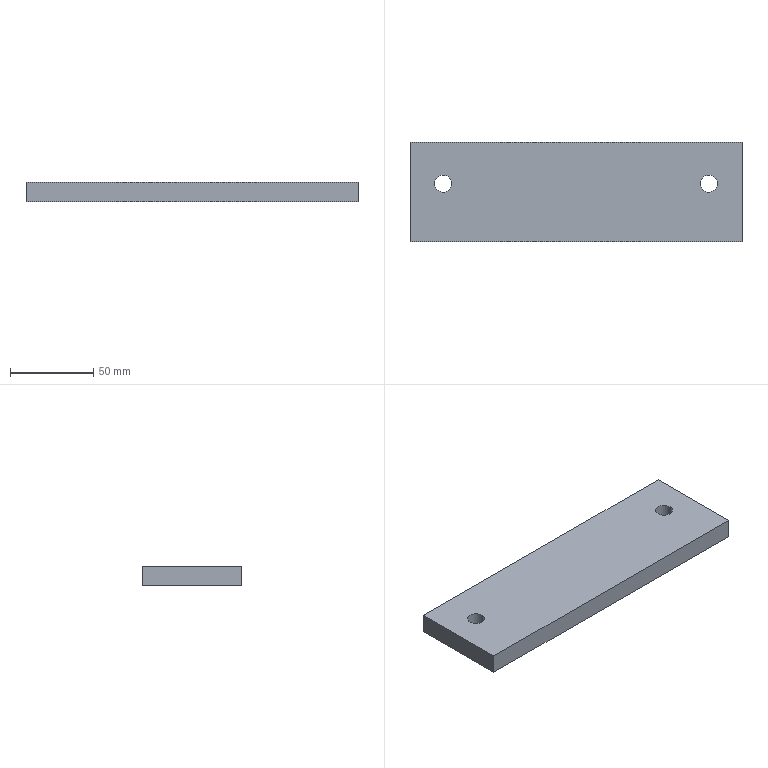Part | SolidWorks | features Extrusion 1, HoleWzd 1 | 1 solid | 10 faces | box 200 x 60 x 12 mm | volume 142039 mm3 | plane 6 | cylinder 4 | commonest cylinder face diameters 10.2 x4
STEP:
#1=CARTESIAN_POINT('',(-85.1,5.,0.));
#2=VERTEX_POINT('',#1);
#3=CARTESIAN_POINT('',(-74.9,5.,0.));
#4=VERTEX_POINT('',#3);
#5=CARTESIAN_POINT('',(-80.,5.,0.));
#6=DIRECTION('',(0.,0.,1.));
#7=DIRECTION('',(1.,0.,0.));
#8=AXIS2_PLACEMENT_3D('',#5,#6,#7);
#9=CIRCLE('',#8,5.1);
#10=EDGE_CURVE('',#2,#4,#9,.T.);
#11=ORIENTED_EDGE('',*,*,#10,.F.);
#12=CARTESIAN_POINT('',(-85.1,5.,12.));
#13=VERTEX_POINT('',#12);
#14=CARTESIAN_POINT('',(-85.1,5.,12.));
#15=DIRECTION('',(0.,0.,1.));
#16=VECTOR('',#15,1000.);
#17=LINE('',#14,#16);
#18=EDGE_CURVE('',#2,#13,#17,.T.);
#19=ORIENTED_EDGE('',*,*,#18,.T.);
#20=CARTESIAN_POINT('',(-74.9,5.,12.));
#21=VERTEX_POINT('',#20);
#22=CARTESIAN_POINT('',(-80.,5.,12.));
#23=DIRECTION('',(0.,0.,1.));
#24=DIRECTION('',(1.,0.,0.));
#25=AXIS2_PLACEMENT_3D('',#22,#23,#24);
#26=CIRCLE('',#25,5.1);
#27=EDGE_CURVE('',#13,#21,#26,.T.);
#28=ORIENTED_EDGE('',*,*,#27,.T.);
#29=CARTESIAN_POINT('',(-74.9,5.,12.));
#30=DIRECTION('',(0.,0.,1.));
#31=VECTOR('',#30,1000.);
#32=LINE('',#29,#31);
#33=EDGE_CURVE('',#4,#21,#32,.T.);
#34=ORIENTED_EDGE('',*,*,#33,.F.);
#35=EDGE_LOOP('',(#11,#19,#28,#34));
#36=FACE_OUTER_BOUND('',#35,.T.);
#37=CARTESIAN_POINT('',(-80.,5.,12.));
#38=DIRECTION('',(0.,0.,1.));
#39=DIRECTION('',(1.,0.,0.));
#40=AXIS2_PLACEMENT_3D('',#37,#38,#39);
#41=CYLINDRICAL_SURFACE('',#40,5.1);
#42=ADVANCED_FACE('',(#36),#41,.F.);
#43=CARTESIAN_POINT('',(74.9,5.,0.));
#44=VERTEX_POINT('',#43);
#45=CARTESIAN_POINT('',(85.1,5.,0.));
#46=VERTEX_POINT('',#45);
#47=CARTESIAN_POINT('',(80.,5.,0.));
#48=DIRECTION('',(0.,0.,1.));
#49=DIRECTION('',(1.,0.,0.));
#50=AXIS2_PLACEMENT_3D('',#47,#48,#49);
#51=CIRCLE('',#50,5.1);
#52=EDGE_CURVE('',#44,#46,#51,.T.);
#53=ORIENTED_EDGE('',*,*,#52,.F.);
#54=CARTESIAN_POINT('',(74.9,5.,12.));
#55=VERTEX_POINT('',#54);
#56=CARTESIAN_POINT('',(74.9,5.,12.));
#57=DIRECTION('',(0.,0.,1.));
#58=VECTOR('',#57,1000.);
#59=LINE('',#56,#58);
#60=EDGE_CURVE('',#44,#55,#59,.T.);
#61=ORIENTED_EDGE('',*,*,#60,.T.);
#62=CARTESIAN_POINT('',(85.1,5.,12.));
#63=VERTEX_POINT('',#62);
#64=CARTESIAN_POINT('',(80.,5.,12.));
#65=DIRECTION('',(0.,0.,1.));
#66=DIRECTION('',(1.,0.,0.));
#67=AXIS2_PLACEMENT_3D('',#64,#65,#66);
#68=CIRCLE('',#67,5.1);
#69=EDGE_CURVE('',#55,#63,#68,.T.);
#70=ORIENTED_EDGE('',*,*,#69,.T.);
#71=CARTESIAN_POINT('',(85.1,5.,12.));
#72=DIRECTION('',(0.,0.,1.));
#73=VECTOR('',#72,1000.);
#74=LINE('',#71,#73);
#75=EDGE_CURVE('',#46,#63,#74,.T.);
#76=ORIENTED_EDGE('',*,*,#75,.F.);
#77=EDGE_LOOP('',(#53,#61,#70,#76));
#78=FACE_OUTER_BOUND('',#77,.T.);
#79=CARTESIAN_POINT('',(80.,5.,12.));
#80=DIRECTION('',(0.,0.,1.));
#81=DIRECTION('',(1.,0.,0.));
#82=AXIS2_PLACEMENT_3D('',#79,#80,#81);
#83=CYLINDRICAL_SURFACE('',#82,5.1);
#84=ADVANCED_FACE('',(#78),#83,.F.);
#85=CARTESIAN_POINT('',(100.,-30.,0.));
#86=VERTEX_POINT('',#85);
#87=CARTESIAN_POINT('',(-100.,-30.,0.));
#88=VERTEX_POINT('',#87);
#89=CARTESIAN_POINT('',(100.,-30.,0.));
#90=DIRECTION('',(-1.,0.,0.));
#91=VECTOR('',#90,1000.);
#92=LINE('',#89,#91);
#93=EDGE_CURVE('',#86,#88,#92,.T.);
#94=ORIENTED_EDGE('',*,*,#93,.F.);
#95=CARTESIAN_POINT('',(100.,-30.,12.));
#96=VERTEX_POINT('',#95);
#97=CARTESIAN_POINT('',(100.,-30.,12.));
#98=DIRECTION('',(0.,0.,-1.));
#99=VECTOR('',#98,1000.);
#100=LINE('',#97,#99);
#101=EDGE_CURVE('',#96,#86,#100,.T.);
#102=ORIENTED_EDGE('',*,*,#101,.F.);
#103=CARTESIAN_POINT('',(-100.,-30.,12.));
#104=VERTEX_POINT('',#103);
#105=CARTESIAN_POINT('',(100.,-30.,12.));
#106=DIRECTION('',(-1.,0.,0.));
#107=VECTOR('',#106,1000.);
#108=LINE('',#105,#107);
#109=EDGE_CURVE('',#96,#104,#108,.T.);
#110=ORIENTED_EDGE('',*,*,#109,.T.);
#111=CARTESIAN_POINT('',(-100.,-30.,12.));
#112=DIRECTION('',(0.,0.,-1.));
#113=VECTOR('',#112,1000.);
#114=LINE('',#111,#113);
#115=EDGE_CURVE('',#104,#88,#114,.T.);
#116=ORIENTED_EDGE('',*,*,#115,.T.);
#117=EDGE_LOOP('',(#94,#102,#110,#116));
#118=FACE_OUTER_BOUND('',#117,.T.);
#119=CARTESIAN_POINT('',(100.,-30.,12.));
#120=DIRECTION('',(0.,-1.,0.));
#121=DIRECTION('',(1.,0.,0.));
#122=AXIS2_PLACEMENT_3D('',#119,#120,#121);
#123=PLANE('',#122);
#124=ADVANCED_FACE('',(#118),#123,.T.);
#125=CARTESIAN_POINT('',(100.,30.,0.));
#126=VERTEX_POINT('',#125);
#127=CARTESIAN_POINT('',(100.,30.,0.));
#128=DIRECTION('',(0.,-1.,0.));
#129=VECTOR('',#128,1000.);
#130=LINE('',#127,#129);
#131=EDGE_CURVE('',#126,#86,#130,.T.);
#132=ORIENTED_EDGE('',*,*,#131,.F.);
#133=CARTESIAN_POINT('',(100.,30.,12.));
#134=VERTEX_POINT('',#133);
#135=CARTESIAN_POINT('',(100.,30.,12.));
#136=DIRECTION('',(0.,0.,-1.));
#137=VECTOR('',#136,1000.);
#138=LINE('',#135,#137);
#139=EDGE_CURVE('',#134,#126,#138,.T.);
#140=ORIENTED_EDGE('',*,*,#139,.F.);
#141=CARTESIAN_POINT('',(100.,30.,12.));
#142=DIRECTION('',(0.,-1.,0.));
#143=VECTOR('',#142,1000.);
#144=LINE('',#141,#143);
#145=EDGE_CURVE('',#134,#96,#144,.T.);
#146=ORIENTED_EDGE('',*,*,#145,.T.);
#147=ORIENTED_EDGE('',*,*,#101,.T.);
#148=EDGE_LOOP('',(#132,#140,#146,#147));
#149=FACE_OUTER_BOUND('',#148,.T.);
#150=CARTESIAN_POINT('',(100.,30.,12.));
#151=DIRECTION('',(1.,0.,0.));
#152=DIRECTION('',(0.,1.,0.));
#153=AXIS2_PLACEMENT_3D('',#150,#151,#152);
#154=PLANE('',#153);
#155=ADVANCED_FACE('',(#149),#154,.T.);
#156=CARTESIAN_POINT('',(-100.,30.,0.));
#157=VERTEX_POINT('',#156);
#158=CARTESIAN_POINT('',(100.,30.,0.));
#159=DIRECTION('',(-1.,0.,0.));
#160=VECTOR('',#159,1000.);
#161=LINE('',#158,#160);
#162=EDGE_CURVE('',#126,#157,#161,.T.);
#163=ORIENTED_EDGE('',*,*,#162,.T.);
#164=CARTESIAN_POINT('',(-100.,30.,12.));
#165=VERTEX_POINT('',#164);
#166=CARTESIAN_POINT('',(-100.,30.,12.));
#167=DIRECTION('',(0.,0.,-1.));
#168=VECTOR('',#167,1000.);
#169=LINE('',#166,#168);
#170=EDGE_CURVE('',#165,#157,#169,.T.);
#171=ORIENTED_EDGE('',*,*,#170,.F.);
#172=CARTESIAN_POINT('',(100.,30.,12.));
#173=DIRECTION('',(-1.,0.,0.));
#174=VECTOR('',#173,1000.);
#175=LINE('',#172,#174);
#176=EDGE_CURVE('',#134,#165,#175,.T.);
#177=ORIENTED_EDGE('',*,*,#176,.F.);
#178=ORIENTED_EDGE('',*,*,#139,.T.);
#179=EDGE_LOOP('',(#163,#171,#177,#178));
#180=FACE_OUTER_BOUND('',#179,.T.);
#181=CARTESIAN_POINT('',(100.,30.,12.));
#182=DIRECTION('',(0.,-1.,0.));
#183=DIRECTION('',(1.,0.,0.));
#184=AXIS2_PLACEMENT_3D('',#181,#182,#183);
#185=PLANE('',#184);
#186=ADVANCED_FACE('',(#180),#185,.F.);
#187=CARTESIAN_POINT('',(-100.,30.,0.));
#188=DIRECTION('',(0.,-1.,0.));
#189=VECTOR('',#188,1000.);
#190=LINE('',#187,#189);
#191=EDGE_CURVE('',#157,#88,#190,.T.);
#192=ORIENTED_EDGE('',*,*,#191,.T.);
#193=ORIENTED_EDGE('',*,*,#115,.F.);
#194=CARTESIAN_POINT('',(-100.,30.,12.));
#195=DIRECTION('',(0.,-1.,0.));
#196=VECTOR('',#195,1000.);
#197=LINE('',#194,#196);
#198=EDGE_CURVE('',#165,#104,#197,.T.);
#199=ORIENTED_EDGE('',*,*,#198,.F.);
#200=ORIENTED_EDGE('',*,*,#170,.T.);
#201=EDGE_LOOP('',(#192,#193,#199,#200));
#202=FACE_OUTER_BOUND('',#201,.T.);
#203=CARTESIAN_POINT('',(-100.,30.,12.));
#204=DIRECTION('',(1.,0.,0.));
#205=DIRECTION('',(0.,1.,0.));
#206=AXIS2_PLACEMENT_3D('',#203,#204,#205);
#207=PLANE('',#206);
#208=ADVANCED_FACE('',(#202),#207,.F.);
#209=CARTESIAN_POINT('',(-80.,5.,12.));
#210=DIRECTION('',(0.,0.,1.));
#211=DIRECTION('',(1.,0.,0.));
#212=AXIS2_PLACEMENT_3D('',#209,#210,#211);
#213=CIRCLE('',#212,5.1);
#214=EDGE_CURVE('',#21,#13,#213,.T.);
#215=ORIENTED_EDGE('',*,*,#214,.F.);
#216=ORIENTED_EDGE('',*,*,#27,.F.);
#217=EDGE_LOOP('',(#215,#216));
#218=FACE_BOUND('',#217,.T.);
#219=CARTESIAN_POINT('',(80.,5.,12.));
#220=DIRECTION('',(0.,0.,1.));
#221=DIRECTION('',(1.,0.,0.));
#222=AXIS2_PLACEMENT_3D('',#219,#220,#221);
#223=CIRCLE('',#222,5.1);
#224=EDGE_CURVE('',#63,#55,#223,.T.);
#225=ORIENTED_EDGE('',*,*,#224,.F.);
#226=ORIENTED_EDGE('',*,*,#69,.F.);
#227=EDGE_LOOP('',(#225,#226));
#228=FACE_BOUND('',#227,.T.);
#229=ORIENTED_EDGE('',*,*,#109,.F.);
#230=ORIENTED_EDGE('',*,*,#145,.F.);
#231=ORIENTED_EDGE('',*,*,#176,.T.);
#232=ORIENTED_EDGE('',*,*,#198,.T.);
#233=EDGE_LOOP('',(#229,#230,#231,#232));
#234=FACE_OUTER_BOUND('',#233,.T.);
#235=CARTESIAN_POINT('',(0.,0.,12.));
#236=DIRECTION('',(0.,0.,1.));
#237=DIRECTION('',(1.,0.,0.));
#238=AXIS2_PLACEMENT_3D('',#235,#236,#237);
#239=PLANE('',#238);
#240=ADVANCED_FACE('',(#218,#228,#234),#239,.T.);
#241=CARTESIAN_POINT('',(-80.,5.,0.));
#242=DIRECTION('',(0.,0.,1.));
#243=DIRECTION('',(1.,0.,0.));
#244=AXIS2_PLACEMENT_3D('',#241,#242,#243);
#245=CIRCLE('',#244,5.1);
#246=EDGE_CURVE('',#4,#2,#245,.T.);
#247=ORIENTED_EDGE('',*,*,#246,.T.);
#248=ORIENTED_EDGE('',*,*,#10,.T.);
#249=EDGE_LOOP('',(#247,#248));
#250=FACE_BOUND('',#249,.T.);
#251=CARTESIAN_POINT('',(80.,5.,0.));
#252=DIRECTION('',(0.,0.,1.));
#253=DIRECTION('',(1.,0.,0.));
#254=AXIS2_PLACEMENT_3D('',#251,#252,#253);
#255=CIRCLE('',#254,5.1);
#256=EDGE_CURVE('',#46,#44,#255,.T.);
#257=ORIENTED_EDGE('',*,*,#256,.T.);
#258=ORIENTED_EDGE('',*,*,#52,.T.);
#259=EDGE_LOOP('',(#257,#258));
#260=FACE_BOUND('',#259,.T.);
#261=ORIENTED_EDGE('',*,*,#93,.T.);
#262=ORIENTED_EDGE('',*,*,#191,.F.);
#263=ORIENTED_EDGE('',*,*,#162,.F.);
#264=ORIENTED_EDGE('',*,*,#131,.T.);
#265=EDGE_LOOP('',(#261,#262,#263,#264));
#266=FACE_OUTER_BOUND('',#265,.T.);
#267=CARTESIAN_POINT('',(0.,0.,0.));
#268=DIRECTION('',(0.,0.,1.));
#269=DIRECTION('',(1.,0.,0.));
#270=AXIS2_PLACEMENT_3D('',#267,#268,#269);
#271=PLANE('',#270);
#272=ADVANCED_FACE('',(#250,#260,#266),#271,.F.);
#273=ORIENTED_EDGE('',*,*,#60,.F.);
#274=ORIENTED_EDGE('',*,*,#256,.F.);
#275=ORIENTED_EDGE('',*,*,#75,.T.);
#276=ORIENTED_EDGE('',*,*,#224,.T.);
#277=EDGE_LOOP('',(#273,#274,#275,#276));
#278=FACE_OUTER_BOUND('',#277,.T.);
#279=CARTESIAN_POINT('',(80.,5.,12.));
#280=DIRECTION('',(0.,0.,1.));
#281=DIRECTION('',(1.,0.,0.));
#282=AXIS2_PLACEMENT_3D('',#279,#280,#281);
#283=CYLINDRICAL_SURFACE('',#282,5.1);
#284=ADVANCED_FACE('',(#278),#283,.F.);
#285=ORIENTED_EDGE('',*,*,#18,.F.);
#286=ORIENTED_EDGE('',*,*,#246,.F.);
#287=ORIENTED_EDGE('',*,*,#33,.T.);
#288=ORIENTED_EDGE('',*,*,#214,.T.);
#289=EDGE_LOOP('',(#285,#286,#287,#288));
#290=FACE_OUTER_BOUND('',#289,.T.);
#291=CARTESIAN_POINT('',(-80.,5.,12.));
#292=DIRECTION('',(0.,0.,1.));
#293=DIRECTION('',(1.,0.,0.));
#294=AXIS2_PLACEMENT_3D('',#291,#292,#293);
#295=CYLINDRICAL_SURFACE('',#294,5.1);
#296=ADVANCED_FACE('',(#290),#295,.F.);
#297=CLOSED_SHELL('',(#42,#84,#124,#155,#186,#208,#240,#272,#284,#296));
#298=MANIFOLD_SOLID_BREP('',#297);
#299=CARTESIAN_POINT('',(0.,0.,0.));
#300=DIRECTION('',(0.,0.,1.));
#301=DIRECTION('',(1.,0.,0.));
#302=AXIS2_PLACEMENT_3D('',#299,#300,#301);
#303=(LENGTH_UNIT()NAMED_UNIT(*)SI_UNIT(.MILLI.,.METRE.));
#304=UNCERTAINTY_MEASURE_WITH_UNIT(LENGTH_MEASURE(0.00001),#303,'','');
#305=(NAMED_UNIT(*)PLANE_ANGLE_UNIT()SI_UNIT($,.RADIAN.));
#306=(NAMED_UNIT(*)SI_UNIT($,.STERADIAN.)SOLID_ANGLE_UNIT());
#307=(GEOMETRIC_REPRESENTATION_CONTEXT(3)GLOBAL_UNCERTAINTY_ASSIGNED_CONTEXT((#304))GLOBAL_UNIT_ASSIGNED_CONTEXT((#303,#305,#306))REPRESENTATION_CONTEXT('',''));
#308=ADVANCED_BREP_SHAPE_REPRESENTATION('',(#298,#302),#307);